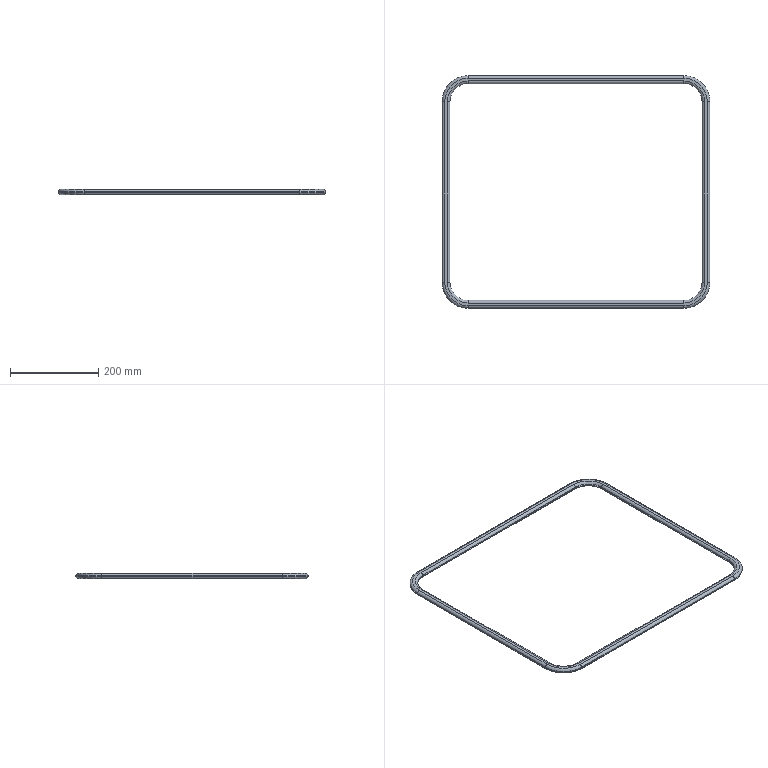Part | STEP file | Part 6^Sheet metal guard | 1 solid | 54 faces | box 607.906 x 527.906 x 12 mm | volume 319171 mm3 | cylinder 24 | torus 16 | plane 14 | commonest cylinder face diameters 12 x16 96 x4 100 x4